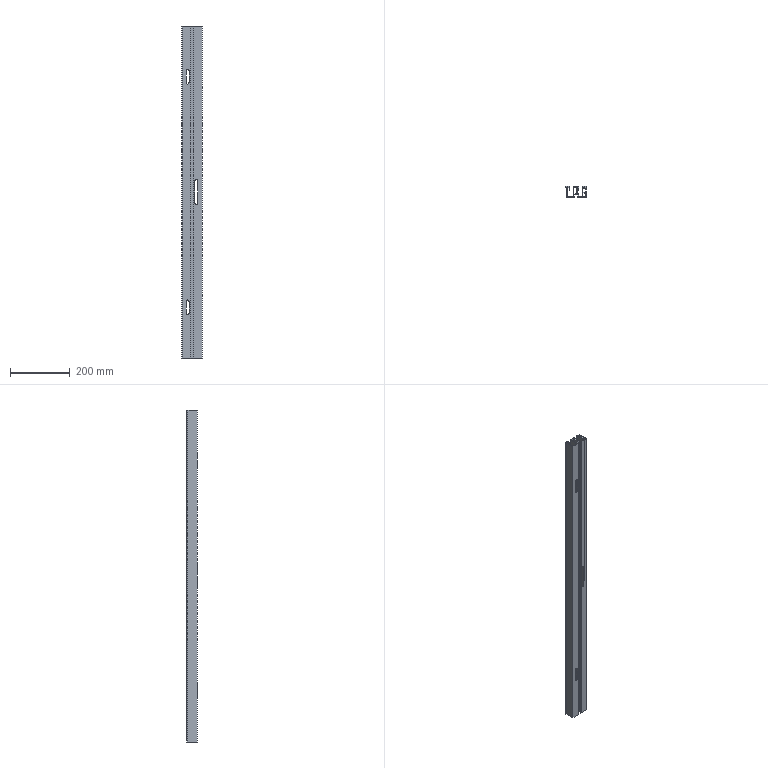Part | 1 solid | 104 faces | box 70 x 35 x 1115 mm | volume 797907 mm3 | plane 68 | cylinder 36 | commonest cylinder face diameters 10 x9 2 x8 6 x8 3 x5 5 x4 1 x1